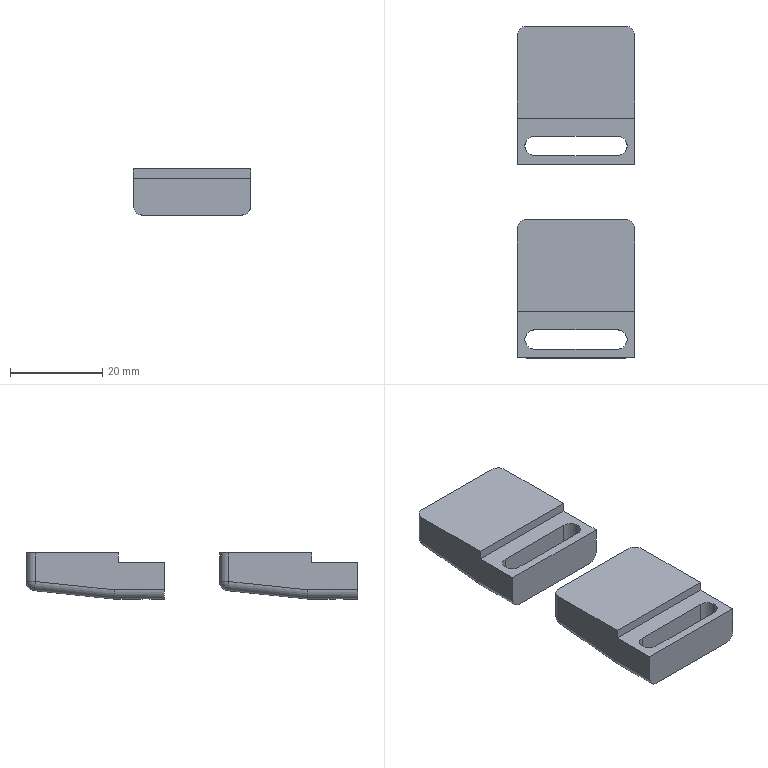NC program | NX | posted with a generic post | part box 25.5 x 72 x 10 mm
Lines 1 to 85 of 60534:
N10 G17 G21 G94 G90
(FLOOR_WALL_COPY_COPY , TOOL : D80)
N12 T19 M6
N14 G54
N16 G17 G0 G90 X83. Y0. B0. C0. S6500 M3
N18 G43 Z30. H19
N20 Z7.
N22 G94 G1 Z4. F1500.
N24 X78.
N26 X-78.
N28 X-83.
N30 Z7.
N32 G0 Z30.
N34 X83.
N36 Z6.
N38 G1 Z3.
N40 X78.
N42 X-78.
N44 X-83.
N46 Z6.
N48 G0 Z30.
N50 X83.
N52 Z5.
N54 G1 Z2.
N56 X78.
N58 X-78.
N60 X-83.
N62 Z5.
N64 G0 Z30.
N66 X83.
N68 Z4.
N70 G1 Z1.
N72 X78.
N74 X-78.
N76 X-83.
N78 Z4.
N80 G0 Z30.
N82 X83.
N84 Z3.
N86 G1 Z0.
N88 X78.
N90 X-78.
N92 X-83.
N94 Z3.
N96 G0 Z30.
N98 M5
(PLANAR_MILL_COPY_COPY_COPY_COPY_COPY_COPY_1_COPY_1_COPY_1 , TOOL : D6A45)
N100 T01 M6
N102 G54
N104 G17 G0 G90 X-10.7 Y0.866 B0. C0. S9500 M3
N106 G43 Z30. H1
N108 Z0.5
N110 G94 G1 Z-1. F1250.
N112 G3 X-11.2 Y0. R1.
N114 G1 Y-9.
N116 G3 X-10. Y-10.2 R1.2
N118 X-8.8 Y-9. R1.2
N120 G1 Y9.
N122 G3 X-10. Y10.2 R1.2
N124 X-11.2 Y9. R1.2
N126 G1 Y0.
N128 G3 X-10.7 Y-0.866 R1.
N130 G1 Z0.5
N132 G0 Z30.
N134 X32.7
N136 Z0.5
N138 G1 Z-1.
N140 G3 X33.2 Y0. R1.
N142 G1 Y9.
N144 G3 X32. Y10.2 R1.2
N146 X30.8 Y9. R1.2
N148 G1 Y-9.
N150 G3 X32. Y-10.2 R1.2
N152 X33.2 Y-9. R1.2
N154 G1 Y0.
N156 G3 X32.7 Y0.866 R1.
N158 G1 Z0.5
N160 G0 Z30.
N162 M5